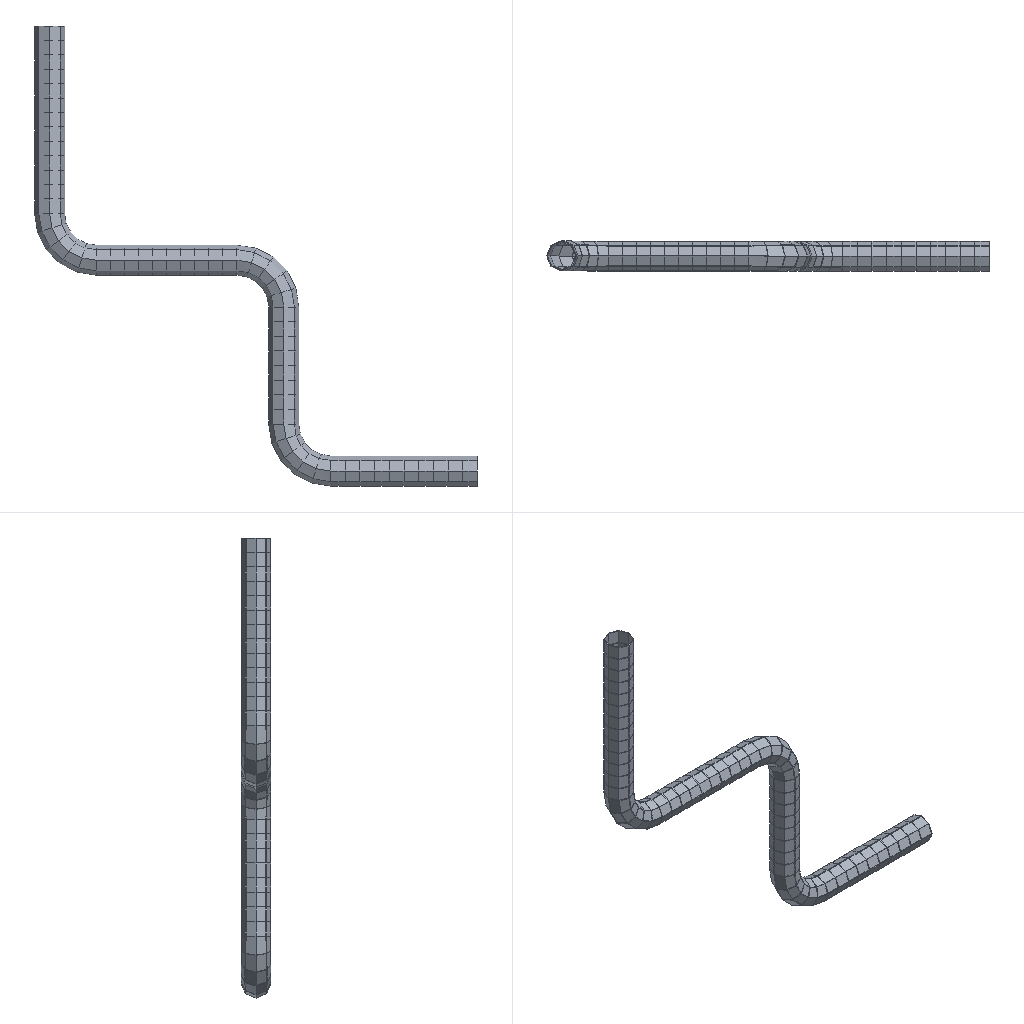Simulation study | abaqus
Set-up summary:
category,name,step,type,value,unit,region
solver,abaqus
solver,version,,,Abaqus/Standard 2020
units,not stated in the deck,,not stated
analysis,deck,,static,static
load_step,Step-1,Step-1,static
load_step,requested,,,1
mesh,nodes,,,912
mesh,elements,,,448
element_type,C3D8R,,solid,448
load,load commands in deck,,count,1
bc,support commands in deck,,count,1
material,MATERIAL-1,,in results
check,setup vs results,,match,"per instance, exact: element labels, types and connectivity; labels of the nodes the elements use; coordinates of those nodes at SINGLE_PRECISION in 1 of 1 instance(s)"
Abaqus input file, long lists of numbers shortened:
*Heading
** Job name: Job-2 Model name: Model-1-Copy
** Generated by: Abaqus/CAE 2020
*Preprint, echo=NO, model=NO, history=NO, contact=NO
**
** PARTS
**
*Part, name=P90
*Node
      1,           0.,         -16.,    151.405
      2,         -16.,           0.,    151.405
** (910 more lines like these left out)
*Element, type=C3D8R
  1,  29,  17,  22,  21,  13,   1,   6,   5
  2,  17,  30,  23,  22,   1,  14,   7,   6
** (446 more lines like these left out)
*Nset, nset=Set-1, generate
   1,  912,    1
*Elset, elset=Set-1, generate
   1,  448,    1
** Section: Section-1
*Solid Section, elset=Set-1, material=Material-1
,
*End Part
**
**
** ASSEMBLY
**
*Assembly, name=Assembly
**
*Instance, name=P90-1, part=P90
*End Instance
**
*Nset, nset=Set-2, instance=P90-1
   1,   2,   3,   4,   5,   6,   7,   8,   9,  10,  11,  12,  13,  14,  15,  16
 897, 898, 899, 900, 901, 902, 903, 904, 905, 906, 907, 908, 909, 910, 911, 912
*Elset, elset=Set-2, instance=P90-1
   1,   2,   3,   4,   5,   6,   7,   8, 441, 442, 443, 444, 445, 446, 447, 448
*Elset, elset=_Surf-2_S3, internal, instance=P90-1
   3,   4,   5,  11,  12,  13,  19,  20,  21,  27,  28,  29,  35,  36,  37,  43
  44,  45,  51,  52,  53,  59,  60,  61,  67,  68,  69,  75,  76,  77,  83,  84
** (9 more lines like these left out)
*Elset, elset=_Surf-2_S5, internal, instance=P90-1
   1,   2,   6,   7,   9,  10,  14,  15,  17,  18,  22,  23,  25,  26,  30,  31
  33,  34,  38,  39,  41,  42,  46,  47,  49,  50,  54,  55,  57,  58,  62,  63
** (12 more lines like these left out)
*Elset, elset=_Surf-2_S6, internal, instance=P90-1, generate
   8,  448,    8
*Surface, type=ELEMENT, name=Surf-2
_Surf-2_S3, S3
_Surf-2_S5, S5
_Surf-2_S6, S6
*End Assembly
*Amplitude, name=Amp-1
             0.,              0.,              1.,              1.
**
** MATERIALS
**
*Material, name=Material-1
*Density
 7.8e-09,
*Elastic
210000., 0.3
*Plastic
350.,0.
** ----------------------------------------------------------------
**
** STEP: Step-1
**
*Step, name=Step-1, nlgeom=YES, inc=1000
*Static, stabilize=0.0002, allsdtol=0.05, continue=NO
0.01, 1., 1e-05, 1.
**
** BOUNDARY CONDITIONS
**
** Name: BC-1 Type: 对称/反对称/完全固定
*Boundary
Set-2, ENCASTRE
**
** LOADS
**
** Name: Load-1   Type: Pressure
*Dsload, amplitude=Amp-1
Surf-2, P, 0.24
**
** OUTPUT REQUESTS
**
*Restart, write, frequency=0
**
** FIELD OUTPUT: F-Output-1
**
*Output, field, variable=PRESELECT
**
** HISTORY OUTPUT: H-Output-1
**
*Output, history, variable=PRESELECT
*End Step
Results summary:
result,step,,completed,increments=11 time=1.0/1.0
result,analysis,,,static
result,last_loadstep,,,1
result,primary field,,,U
result,reaction total,,FX,152.624,model units
result,reaction total,,FY,-0.0,model units
result,reaction total,,FZ,152.674,model units